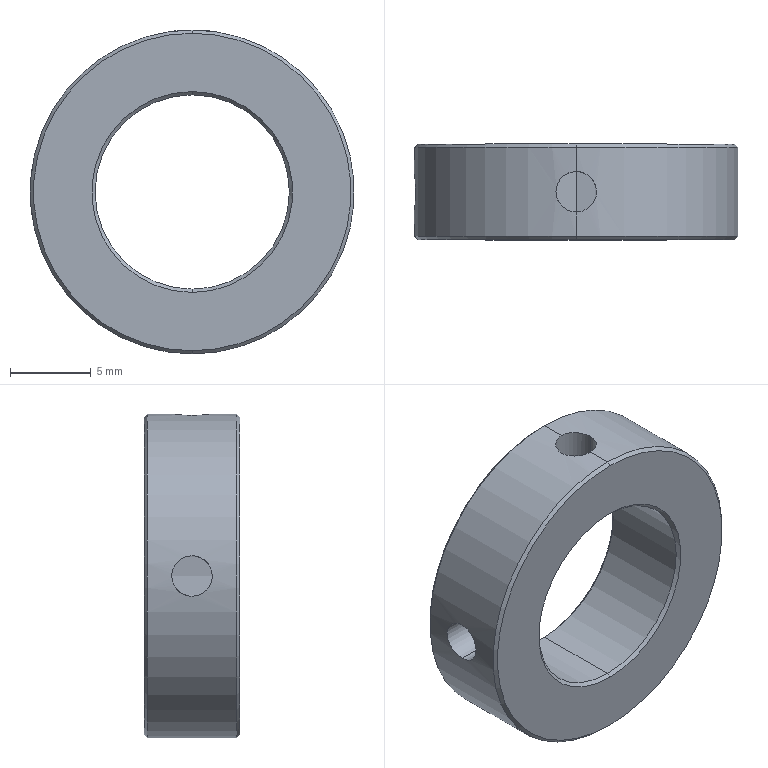Part | STEP file | ND25021-01-JDKM-08-GJ | 1 solid | 18 faces | box 20 x 5.9 x 20 mm | volume 1143 mm3 | cone 8 | cylinder 8 | plane 2 | commonest cylinder face diameters 2.5 x4 12 x2 20 x2